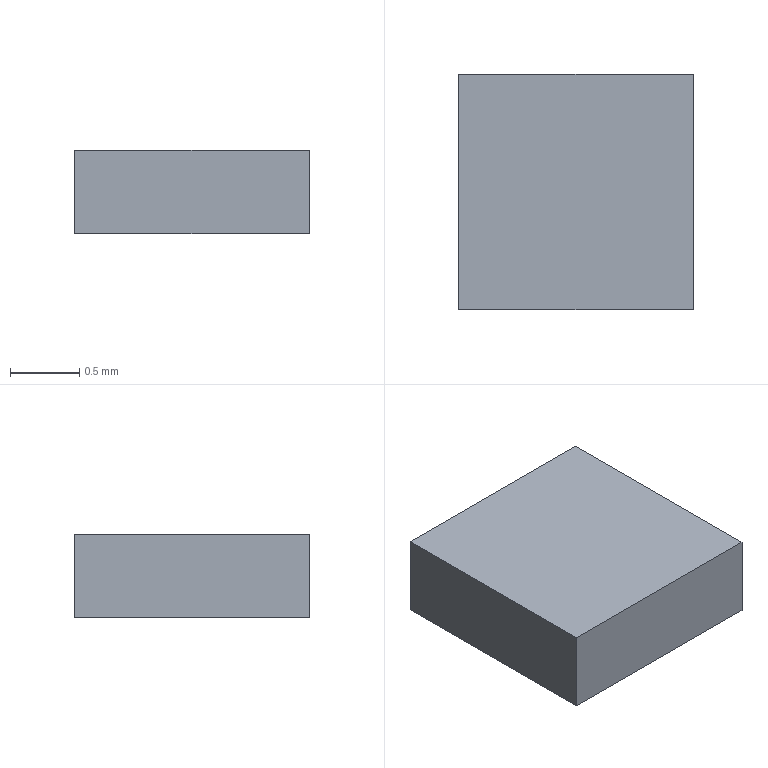Part | Creo | 1 solid | 6 faces | box 1.685 x 1.694 x 0.6 mm | volume 1.713 mm3 | plane 6
STEP:
#1=CARTESIAN_POINT('',(0.,0.,0.));
#2=DIRECTION('',(0.,0.,1.));
#3=DIRECTION('',(1.,0.,0.));
#4=AXIS2_PLACEMENT_3D('',#1,#2,#3);
#5=CARTESIAN_POINT('',(-0.885,-0.8,0.));
#6=VERTEX_POINT('',#5);
#7=CARTESIAN_POINT('',(0.8,-0.8,0.));
#8=VERTEX_POINT('',#7);
#9=CARTESIAN_POINT('',(-0.885,-0.8,0.));
#10=DIRECTION('',(1.,0.,0.));
#11=VECTOR('',#10,1.685);
#12=LINE('',#9,#11);
#13=EDGE_CURVE('',#6,#8,#12,.T.);
#14=ORIENTED_EDGE('',*,*,#13,.T.);
#15=CARTESIAN_POINT('',(0.8,0.894,0.));
#16=VERTEX_POINT('',#15);
#17=CARTESIAN_POINT('',(0.8,-0.8,0.));
#18=DIRECTION('',(0.,1.,0.));
#19=VECTOR('',#18,1.694);
#20=LINE('',#17,#19);
#21=EDGE_CURVE('',#8,#16,#20,.T.);
#22=ORIENTED_EDGE('',*,*,#21,.T.);
#23=CARTESIAN_POINT('',(-0.885,0.894,0.));
#24=VERTEX_POINT('',#23);
#25=CARTESIAN_POINT('',(0.8,0.894,0.));
#26=DIRECTION('',(-1.,0.,0.));
#27=VECTOR('',#26,1.685);
#28=LINE('',#25,#27);
#29=EDGE_CURVE('',#16,#24,#28,.T.);
#30=ORIENTED_EDGE('',*,*,#29,.T.);
#31=CARTESIAN_POINT('',(-0.885,0.894,0.));
#32=DIRECTION('',(0.,-1.,0.));
#33=VECTOR('',#32,1.694);
#34=LINE('',#31,#33);
#35=EDGE_CURVE('',#24,#6,#34,.T.);
#36=ORIENTED_EDGE('',*,*,#35,.T.);
#37=EDGE_LOOP('',(#14,#22,#30,#36));
#38=FACE_OUTER_BOUND('',#37,.F.);
#39=CARTESIAN_POINT('',(0.,0.,0.));
#40=DIRECTION('',(0.,0.,1.));
#41=DIRECTION('',(1.,0.,0.));
#42=AXIS2_PLACEMENT_3D('',#39,#40,#41);
#43=PLANE('',#42);
#44=ADVANCED_FACE('',(#38),#43,.F.);
#45=ORIENTED_EDGE('',*,*,#13,.F.);
#46=CARTESIAN_POINT('',(-0.885,-0.8,0.6));
#47=VERTEX_POINT('',#46);
#48=CARTESIAN_POINT('',(-0.885,-0.8,0.));
#49=DIRECTION('',(0.,0.,1.));
#50=VECTOR('',#49,0.6);
#51=LINE('',#48,#50);
#52=EDGE_CURVE('',#6,#47,#51,.T.);
#53=ORIENTED_EDGE('',*,*,#52,.T.);
#54=CARTESIAN_POINT('',(0.8,-0.8,0.6));
#55=VERTEX_POINT('',#54);
#56=CARTESIAN_POINT('',(-0.885,-0.8,0.6));
#57=DIRECTION('',(1.,0.,0.));
#58=VECTOR('',#57,1.685);
#59=LINE('',#56,#58);
#60=EDGE_CURVE('',#47,#55,#59,.T.);
#61=ORIENTED_EDGE('',*,*,#60,.T.);
#62=CARTESIAN_POINT('',(0.8,-0.8,0.));
#63=DIRECTION('',(0.,0.,1.));
#64=VECTOR('',#63,0.6);
#65=LINE('',#62,#64);
#66=EDGE_CURVE('',#8,#55,#65,.T.);
#67=ORIENTED_EDGE('',*,*,#66,.F.);
#68=EDGE_LOOP('',(#45,#53,#61,#67));
#69=FACE_OUTER_BOUND('',#68,.F.);
#70=CARTESIAN_POINT('',(-0.885,-0.8,0.));
#71=DIRECTION('',(0.,-1.,0.));
#72=DIRECTION('',(1.,0.,0.));
#73=AXIS2_PLACEMENT_3D('',#70,#71,#72);
#74=PLANE('',#73);
#75=ADVANCED_FACE('',(#69),#74,.T.);
#76=ORIENTED_EDGE('',*,*,#35,.F.);
#77=CARTESIAN_POINT('',(-0.885,0.894,0.6));
#78=VERTEX_POINT('',#77);
#79=CARTESIAN_POINT('',(-0.885,0.894,0.));
#80=DIRECTION('',(0.,0.,1.));
#81=VECTOR('',#80,0.6);
#82=LINE('',#79,#81);
#83=EDGE_CURVE('',#24,#78,#82,.T.);
#84=ORIENTED_EDGE('',*,*,#83,.T.);
#85=CARTESIAN_POINT('',(-0.885,0.894,0.6));
#86=DIRECTION('',(0.,-1.,0.));
#87=VECTOR('',#86,1.694);
#88=LINE('',#85,#87);
#89=EDGE_CURVE('',#78,#47,#88,.T.);
#90=ORIENTED_EDGE('',*,*,#89,.T.);
#91=ORIENTED_EDGE('',*,*,#52,.F.);
#92=EDGE_LOOP('',(#76,#84,#90,#91));
#93=FACE_OUTER_BOUND('',#92,.F.);
#94=CARTESIAN_POINT('',(-0.885,0.894,0.));
#95=DIRECTION('',(-1.,0.,0.));
#96=DIRECTION('',(0.,-1.,0.));
#97=AXIS2_PLACEMENT_3D('',#94,#95,#96);
#98=PLANE('',#97);
#99=ADVANCED_FACE('',(#93),#98,.T.);
#100=ORIENTED_EDGE('',*,*,#29,.F.);
#101=CARTESIAN_POINT('',(0.8,0.894,0.6));
#102=VERTEX_POINT('',#101);
#103=CARTESIAN_POINT('',(0.8,0.894,0.));
#104=DIRECTION('',(0.,0.,1.));
#105=VECTOR('',#104,0.6);
#106=LINE('',#103,#105);
#107=EDGE_CURVE('',#16,#102,#106,.T.);
#108=ORIENTED_EDGE('',*,*,#107,.T.);
#109=CARTESIAN_POINT('',(0.8,0.894,0.6));
#110=DIRECTION('',(-1.,0.,0.));
#111=VECTOR('',#110,1.685);
#112=LINE('',#109,#111);
#113=EDGE_CURVE('',#102,#78,#112,.T.);
#114=ORIENTED_EDGE('',*,*,#113,.T.);
#115=ORIENTED_EDGE('',*,*,#83,.F.);
#116=EDGE_LOOP('',(#100,#108,#114,#115));
#117=FACE_OUTER_BOUND('',#116,.F.);
#118=CARTESIAN_POINT('',(0.8,0.894,0.));
#119=DIRECTION('',(0.,1.,0.));
#120=DIRECTION('',(-1.,0.,0.));
#121=AXIS2_PLACEMENT_3D('',#118,#119,#120);
#122=PLANE('',#121);
#123=ADVANCED_FACE('',(#117),#122,.T.);
#124=ORIENTED_EDGE('',*,*,#21,.F.);
#125=ORIENTED_EDGE('',*,*,#66,.T.);
#126=CARTESIAN_POINT('',(0.8,-0.8,0.6));
#127=DIRECTION('',(0.,1.,0.));
#128=VECTOR('',#127,1.694);
#129=LINE('',#126,#128);
#130=EDGE_CURVE('',#55,#102,#129,.T.);
#131=ORIENTED_EDGE('',*,*,#130,.T.);
#132=ORIENTED_EDGE('',*,*,#107,.F.);
#133=EDGE_LOOP('',(#124,#125,#131,#132));
#134=FACE_OUTER_BOUND('',#133,.F.);
#135=CARTESIAN_POINT('',(0.8,-0.8,0.));
#136=DIRECTION('',(1.,0.,0.));
#137=DIRECTION('',(0.,1.,0.));
#138=AXIS2_PLACEMENT_3D('',#135,#136,#137);
#139=PLANE('',#138);
#140=ADVANCED_FACE('',(#134),#139,.T.);
#141=ORIENTED_EDGE('',*,*,#60,.F.);
#142=ORIENTED_EDGE('',*,*,#89,.F.);
#143=ORIENTED_EDGE('',*,*,#113,.F.);
#144=ORIENTED_EDGE('',*,*,#130,.F.);
#145=EDGE_LOOP('',(#141,#142,#143,#144));
#146=FACE_OUTER_BOUND('',#145,.F.);
#147=CARTESIAN_POINT('',(0.,0.,0.6));
#148=DIRECTION('',(0.,0.,1.));
#149=DIRECTION('',(1.,0.,0.));
#150=AXIS2_PLACEMENT_3D('',#147,#148,#149);
#151=PLANE('',#150);
#152=ADVANCED_FACE('',(#146),#151,.T.);
#153=CLOSED_SHELL('',(#44,#75,#99,#123,#140,#152));
#154=MANIFOLD_SOLID_BREP('',#153);
#155=(LENGTH_UNIT()NAMED_UNIT(*)SI_UNIT(.MILLI.,.METRE.));
#156=UNCERTAINTY_MEASURE_WITH_UNIT(LENGTH_MEASURE(0.0002463),#155,'','');
#157=(NAMED_UNIT(*)PLANE_ANGLE_UNIT()SI_UNIT($,.RADIAN.));
#158=PLANE_ANGLE_MEASURE_WITH_UNIT(PLANE_ANGLE_MEASURE(0.01745),#157);
#159=(CONVERSION_BASED_UNIT('DEGREE',#158)NAMED_UNIT(*)PLANE_ANGLE_UNIT());
#160=(NAMED_UNIT(*)SI_UNIT($,.STERADIAN.)SOLID_ANGLE_UNIT());
#161=(GEOMETRIC_REPRESENTATION_CONTEXT(3)GLOBAL_UNCERTAINTY_ASSIGNED_CONTEXT((#156))GLOBAL_UNIT_ASSIGNED_CONTEXT((#155,#159,#160))REPRESENTATION_CONTEXT('',''));
#162=ADVANCED_BREP_SHAPE_REPRESENTATION('',(#4,#154),#161);